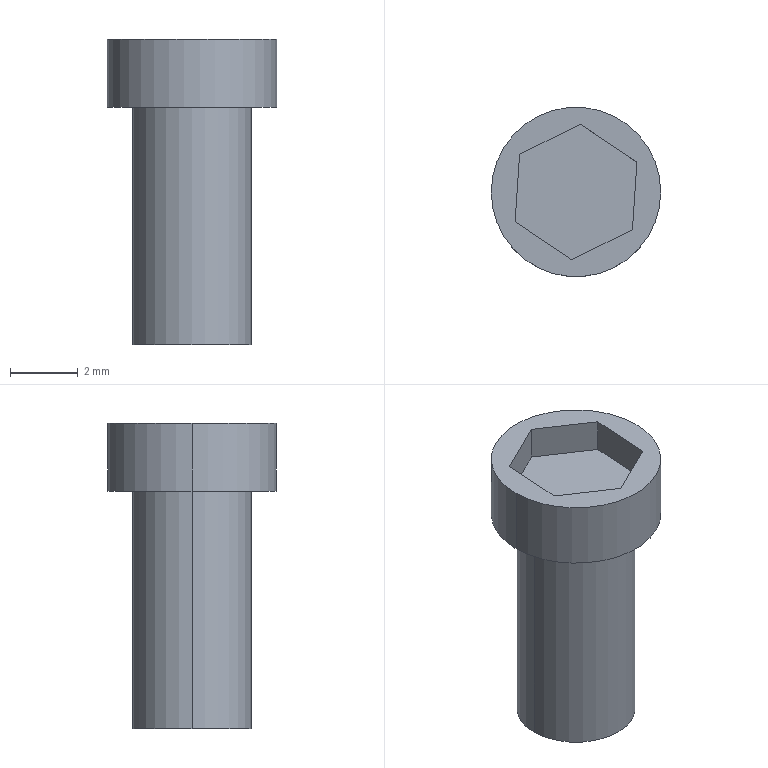Part | SolidWorks | features ICE 2, Extrusion 1 | 1 solid | 14 faces | box 5 x 5 x 9 mm | volume 96.197 mm3 | plane 10 | cylinder 4 | commonest cylinder face diameters 3.5 x2 5 x2
STEP:
#1=CARTESIAN_POINT('',(-1.75,0.,-7.));
#2=VERTEX_POINT('',#1);
#3=CARTESIAN_POINT('',(1.75,0.,-7.));
#4=VERTEX_POINT('',#3);
#5=CARTESIAN_POINT('',(0.,0.,-7.));
#6=DIRECTION('',(0.,0.,-1.));
#7=DIRECTION('',(-1.,0.,0.));
#8=AXIS2_PLACEMENT_3D('',#5,#6,#7);
#9=CIRCLE('',#8,1.75);
#10=EDGE_CURVE('',#2,#4,#9,.T.);
#11=ORIENTED_EDGE('',*,*,#10,.F.);
#12=CARTESIAN_POINT('',(-1.75,0.,0.));
#13=VERTEX_POINT('',#12);
#14=CARTESIAN_POINT('',(-1.75,0.,-7.));
#15=DIRECTION('',(0.,0.,1.));
#16=VECTOR('',#15,1000.);
#17=LINE('',#14,#16);
#18=EDGE_CURVE('',#2,#13,#17,.T.);
#19=ORIENTED_EDGE('',*,*,#18,.T.);
#20=CARTESIAN_POINT('',(1.75,0.,0.));
#21=VERTEX_POINT('',#20);
#22=CARTESIAN_POINT('',(0.,0.,0.));
#23=DIRECTION('',(0.,0.,-1.));
#24=DIRECTION('',(-1.,0.,0.));
#25=AXIS2_PLACEMENT_3D('',#22,#23,#24);
#26=CIRCLE('',#25,1.75);
#27=EDGE_CURVE('',#13,#21,#26,.T.);
#28=ORIENTED_EDGE('',*,*,#27,.T.);
#29=CARTESIAN_POINT('',(1.75,0.,-7.));
#30=DIRECTION('',(0.,0.,1.));
#31=VECTOR('',#30,1000.);
#32=LINE('',#29,#31);
#33=EDGE_CURVE('',#4,#21,#32,.T.);
#34=ORIENTED_EDGE('',*,*,#33,.F.);
#35=EDGE_LOOP('',(#11,#19,#28,#34));
#36=FACE_OUTER_BOUND('',#35,.T.);
#37=CARTESIAN_POINT('',(0.,0.,-7.));
#38=DIRECTION('',(0.,0.,1.));
#39=DIRECTION('',(1.,0.,0.));
#40=AXIS2_PLACEMENT_3D('',#37,#38,#39);
#41=CYLINDRICAL_SURFACE('',#40,1.75);
#42=ADVANCED_FACE('',(#36),#41,.T.);
#43=CARTESIAN_POINT('',(2.5,0.,2.));
#44=VERTEX_POINT('',#43);
#45=CARTESIAN_POINT('',(-2.5,0.,2.));
#46=VERTEX_POINT('',#45);
#47=CARTESIAN_POINT('',(0.,0.,2.));
#48=DIRECTION('',(0.,0.,1.));
#49=DIRECTION('',(1.,0.,0.));
#50=AXIS2_PLACEMENT_3D('',#47,#48,#49);
#51=CIRCLE('',#50,2.5);
#52=EDGE_CURVE('',#44,#46,#51,.T.);
#53=ORIENTED_EDGE('',*,*,#52,.F.);
#54=CARTESIAN_POINT('',(2.5,0.,0.));
#55=VERTEX_POINT('',#54);
#56=CARTESIAN_POINT('',(2.5,0.,2.));
#57=DIRECTION('',(0.,0.,-1.));
#58=VECTOR('',#57,1000.);
#59=LINE('',#56,#58);
#60=EDGE_CURVE('',#44,#55,#59,.T.);
#61=ORIENTED_EDGE('',*,*,#60,.T.);
#62=CARTESIAN_POINT('',(-2.5,0.,0.));
#63=VERTEX_POINT('',#62);
#64=CARTESIAN_POINT('',(0.,0.,0.));
#65=DIRECTION('',(0.,0.,1.));
#66=DIRECTION('',(1.,0.,0.));
#67=AXIS2_PLACEMENT_3D('',#64,#65,#66);
#68=CIRCLE('',#67,2.5);
#69=EDGE_CURVE('',#55,#63,#68,.T.);
#70=ORIENTED_EDGE('',*,*,#69,.T.);
#71=CARTESIAN_POINT('',(-2.5,0.,2.));
#72=DIRECTION('',(0.,0.,-1.));
#73=VECTOR('',#72,1000.);
#74=LINE('',#71,#73);
#75=EDGE_CURVE('',#46,#63,#74,.T.);
#76=ORIENTED_EDGE('',*,*,#75,.F.);
#77=EDGE_LOOP('',(#53,#61,#70,#76));
#78=FACE_OUTER_BOUND('',#77,.T.);
#79=CARTESIAN_POINT('',(0.,0.,2.));
#80=DIRECTION('',(0.,0.,-1.));
#81=DIRECTION('',(-1.,0.,0.));
#82=AXIS2_PLACEMENT_3D('',#79,#80,#81);
#83=CYLINDRICAL_SURFACE('',#82,2.5);
#84=ADVANCED_FACE('',(#78),#83,.T.);
#85=ORIENTED_EDGE('',*,*,#60,.F.);
#86=CARTESIAN_POINT('',(0.,0.,2.));
#87=DIRECTION('',(0.,0.,1.));
#88=DIRECTION('',(1.,0.,0.));
#89=AXIS2_PLACEMENT_3D('',#86,#87,#88);
#90=CIRCLE('',#89,2.5);
#91=EDGE_CURVE('',#46,#44,#90,.T.);
#92=ORIENTED_EDGE('',*,*,#91,.F.);
#93=ORIENTED_EDGE('',*,*,#75,.T.);
#94=CARTESIAN_POINT('',(0.,0.,0.));
#95=DIRECTION('',(0.,0.,1.));
#96=DIRECTION('',(1.,0.,0.));
#97=AXIS2_PLACEMENT_3D('',#94,#95,#96);
#98=CIRCLE('',#97,2.5);
#99=EDGE_CURVE('',#63,#55,#98,.T.);
#100=ORIENTED_EDGE('',*,*,#99,.T.);
#101=EDGE_LOOP('',(#85,#92,#93,#100));
#102=FACE_OUTER_BOUND('',#101,.T.);
#103=CARTESIAN_POINT('',(0.,0.,2.));
#104=DIRECTION('',(0.,0.,-1.));
#105=DIRECTION('',(-1.,0.,0.));
#106=AXIS2_PLACEMENT_3D('',#103,#104,#105);
#107=CYLINDRICAL_SURFACE('',#106,2.5);
#108=ADVANCED_FACE('',(#102),#107,.T.);
#109=CARTESIAN_POINT('',(-0.1337,-1.998,2.));
#110=VERTEX_POINT('',#109);
#111=CARTESIAN_POINT('',(1.664,-1.115,2.));
#112=VERTEX_POINT('',#111);
#113=CARTESIAN_POINT('',(-0.1337,-1.998,2.));
#114=DIRECTION('',(0.8975,0.4411,0.));
#115=VECTOR('',#114,1000.);
#116=LINE('',#113,#115);
#117=EDGE_CURVE('',#110,#112,#116,.T.);
#118=ORIENTED_EDGE('',*,*,#117,.F.);
#119=CARTESIAN_POINT('',(-1.797,-0.8833,2.));
#120=VERTEX_POINT('',#119);
#121=CARTESIAN_POINT('',(-1.797,-0.8833,2.));
#122=DIRECTION('',(0.8307,-0.5567,0.));
#123=VECTOR('',#122,1000.);
#124=LINE('',#121,#123);
#125=EDGE_CURVE('',#120,#110,#124,.T.);
#126=ORIENTED_EDGE('',*,*,#125,.F.);
#127=CARTESIAN_POINT('',(-1.664,1.115,2.));
#128=VERTEX_POINT('',#127);
#129=CARTESIAN_POINT('',(-1.664,1.115,2.));
#130=DIRECTION('',(-0.06677,-0.9978,0.));
#131=VECTOR('',#130,1000.);
#132=LINE('',#129,#131);
#133=EDGE_CURVE('',#128,#120,#132,.T.);
#134=ORIENTED_EDGE('',*,*,#133,.F.);
#135=CARTESIAN_POINT('',(0.1337,1.998,2.));
#136=VERTEX_POINT('',#135);
#137=CARTESIAN_POINT('',(0.1337,1.998,2.));
#138=DIRECTION('',(-0.8975,-0.4411,0.));
#139=VECTOR('',#138,1000.);
#140=LINE('',#137,#139);
#141=EDGE_CURVE('',#136,#128,#140,.T.);
#142=ORIENTED_EDGE('',*,*,#141,.F.);
#143=CARTESIAN_POINT('',(1.797,0.8833,2.));
#144=VERTEX_POINT('',#143);
#145=CARTESIAN_POINT('',(1.797,0.8833,2.));
#146=DIRECTION('',(-0.8307,0.5567,0.));
#147=VECTOR('',#146,1000.);
#148=LINE('',#145,#147);
#149=EDGE_CURVE('',#144,#136,#148,.T.);
#150=ORIENTED_EDGE('',*,*,#149,.F.);
#151=CARTESIAN_POINT('',(1.664,-1.115,2.));
#152=DIRECTION('',(0.06677,0.9978,0.));
#153=VECTOR('',#152,1000.);
#154=LINE('',#151,#153);
#155=EDGE_CURVE('',#112,#144,#154,.T.);
#156=ORIENTED_EDGE('',*,*,#155,.F.);
#157=EDGE_LOOP('',(#118,#126,#134,#142,#150,#156));
#158=FACE_BOUND('',#157,.T.);
#159=ORIENTED_EDGE('',*,*,#91,.T.);
#160=ORIENTED_EDGE('',*,*,#52,.T.);
#161=EDGE_LOOP('',(#159,#160));
#162=FACE_OUTER_BOUND('',#161,.T.);
#163=CARTESIAN_POINT('',(0.,0.,2.));
#164=DIRECTION('',(0.,0.,1.));
#165=DIRECTION('',(1.,0.,0.));
#166=AXIS2_PLACEMENT_3D('',#163,#164,#165);
#167=PLANE('',#166);
#168=ADVANCED_FACE('',(#158,#162),#167,.T.);
#169=CARTESIAN_POINT('',(0.,0.,0.));
#170=DIRECTION('',(0.,0.,-1.));
#171=DIRECTION('',(-1.,0.,0.));
#172=AXIS2_PLACEMENT_3D('',#169,#170,#171);
#173=CIRCLE('',#172,1.75);
#174=EDGE_CURVE('',#21,#13,#173,.T.);
#175=ORIENTED_EDGE('',*,*,#174,.F.);
#176=ORIENTED_EDGE('',*,*,#27,.F.);
#177=EDGE_LOOP('',(#175,#176));
#178=FACE_BOUND('',#177,.T.);
#179=ORIENTED_EDGE('',*,*,#99,.F.);
#180=ORIENTED_EDGE('',*,*,#69,.F.);
#181=EDGE_LOOP('',(#179,#180));
#182=FACE_OUTER_BOUND('',#181,.T.);
#183=CARTESIAN_POINT('',(0.,0.,0.));
#184=DIRECTION('',(0.,0.,1.));
#185=DIRECTION('',(1.,0.,0.));
#186=AXIS2_PLACEMENT_3D('',#183,#184,#185);
#187=PLANE('',#186);
#188=ADVANCED_FACE('',(#178,#182),#187,.F.);
#189=ORIENTED_EDGE('',*,*,#117,.T.);
#190=CARTESIAN_POINT('',(1.664,-1.115,1.));
#191=VERTEX_POINT('',#190);
#192=CARTESIAN_POINT('',(1.664,-1.115,1.));
#193=DIRECTION('',(0.,0.,1.));
#194=VECTOR('',#193,1000.);
#195=LINE('',#192,#194);
#196=EDGE_CURVE('',#191,#112,#195,.T.);
#197=ORIENTED_EDGE('',*,*,#196,.F.);
#198=CARTESIAN_POINT('',(-0.1337,-1.998,1.));
#199=VERTEX_POINT('',#198);
#200=CARTESIAN_POINT('',(-0.1337,-1.998,1.));
#201=DIRECTION('',(0.8975,0.4411,0.));
#202=VECTOR('',#201,1000.);
#203=LINE('',#200,#202);
#204=EDGE_CURVE('',#199,#191,#203,.T.);
#205=ORIENTED_EDGE('',*,*,#204,.F.);
#206=CARTESIAN_POINT('',(-0.1337,-1.998,1.));
#207=DIRECTION('',(0.,0.,1.));
#208=VECTOR('',#207,1000.);
#209=LINE('',#206,#208);
#210=EDGE_CURVE('',#199,#110,#209,.T.);
#211=ORIENTED_EDGE('',*,*,#210,.T.);
#212=EDGE_LOOP('',(#189,#197,#205,#211));
#213=FACE_OUTER_BOUND('',#212,.T.);
#214=CARTESIAN_POINT('',(-0.1337,-1.998,1.));
#215=DIRECTION('',(0.4411,-0.8975,0.));
#216=DIRECTION('',(0.8975,0.4411,0.));
#217=AXIS2_PLACEMENT_3D('',#214,#215,#216);
#218=PLANE('',#217);
#219=ADVANCED_FACE('',(#213),#218,.F.);
#220=ORIENTED_EDGE('',*,*,#125,.T.);
#221=ORIENTED_EDGE('',*,*,#210,.F.);
#222=CARTESIAN_POINT('',(-1.797,-0.8833,1.));
#223=VERTEX_POINT('',#222);
#224=CARTESIAN_POINT('',(-1.797,-0.8833,1.));
#225=DIRECTION('',(0.8307,-0.5567,0.));
#226=VECTOR('',#225,1000.);
#227=LINE('',#224,#226);
#228=EDGE_CURVE('',#223,#199,#227,.T.);
#229=ORIENTED_EDGE('',*,*,#228,.F.);
#230=CARTESIAN_POINT('',(-1.797,-0.8833,1.));
#231=DIRECTION('',(0.,0.,1.));
#232=VECTOR('',#231,1000.);
#233=LINE('',#230,#232);
#234=EDGE_CURVE('',#223,#120,#233,.T.);
#235=ORIENTED_EDGE('',*,*,#234,.T.);
#236=EDGE_LOOP('',(#220,#221,#229,#235));
#237=FACE_OUTER_BOUND('',#236,.T.);
#238=CARTESIAN_POINT('',(-1.797,-0.8833,1.));
#239=DIRECTION('',(-0.5567,-0.8307,0.));
#240=DIRECTION('',(0.8307,-0.5567,0.));
#241=AXIS2_PLACEMENT_3D('',#238,#239,#240);
#242=PLANE('',#241);
#243=ADVANCED_FACE('',(#237),#242,.F.);
#244=ORIENTED_EDGE('',*,*,#133,.T.);
#245=ORIENTED_EDGE('',*,*,#234,.F.);
#246=CARTESIAN_POINT('',(-1.664,1.115,1.));
#247=VERTEX_POINT('',#246);
#248=CARTESIAN_POINT('',(-1.664,1.115,1.));
#249=DIRECTION('',(-0.06677,-0.9978,0.));
#250=VECTOR('',#249,1000.);
#251=LINE('',#248,#250);
#252=EDGE_CURVE('',#247,#223,#251,.T.);
#253=ORIENTED_EDGE('',*,*,#252,.F.);
#254=CARTESIAN_POINT('',(-1.664,1.115,1.));
#255=DIRECTION('',(0.,0.,1.));
#256=VECTOR('',#255,1000.);
#257=LINE('',#254,#256);
#258=EDGE_CURVE('',#247,#128,#257,.T.);
#259=ORIENTED_EDGE('',*,*,#258,.T.);
#260=EDGE_LOOP('',(#244,#245,#253,#259));
#261=FACE_OUTER_BOUND('',#260,.T.);
#262=CARTESIAN_POINT('',(-1.664,1.115,1.));
#263=DIRECTION('',(-0.9978,0.06677,0.));
#264=DIRECTION('',(-0.06677,-0.9978,0.));
#265=AXIS2_PLACEMENT_3D('',#262,#263,#264);
#266=PLANE('',#265);
#267=ADVANCED_FACE('',(#261),#266,.F.);
#268=ORIENTED_EDGE('',*,*,#141,.T.);
#269=ORIENTED_EDGE('',*,*,#258,.F.);
#270=CARTESIAN_POINT('',(0.1337,1.998,1.));
#271=VERTEX_POINT('',#270);
#272=CARTESIAN_POINT('',(0.1337,1.998,1.));
#273=DIRECTION('',(-0.8975,-0.4411,0.));
#274=VECTOR('',#273,1000.);
#275=LINE('',#272,#274);
#276=EDGE_CURVE('',#271,#247,#275,.T.);
#277=ORIENTED_EDGE('',*,*,#276,.F.);
#278=CARTESIAN_POINT('',(0.1337,1.998,1.));
#279=DIRECTION('',(0.,0.,1.));
#280=VECTOR('',#279,1000.);
#281=LINE('',#278,#280);
#282=EDGE_CURVE('',#271,#136,#281,.T.);
#283=ORIENTED_EDGE('',*,*,#282,.T.);
#284=EDGE_LOOP('',(#268,#269,#277,#283));
#285=FACE_OUTER_BOUND('',#284,.T.);
#286=CARTESIAN_POINT('',(0.1337,1.998,1.));
#287=DIRECTION('',(-0.4411,0.8975,0.));
#288=DIRECTION('',(-0.8975,-0.4411,0.));
#289=AXIS2_PLACEMENT_3D('',#286,#287,#288);
#290=PLANE('',#289);
#291=ADVANCED_FACE('',(#285),#290,.F.);
#292=ORIENTED_EDGE('',*,*,#149,.T.);
#293=ORIENTED_EDGE('',*,*,#282,.F.);
#294=CARTESIAN_POINT('',(1.797,0.8833,1.));
#295=VERTEX_POINT('',#294);
#296=CARTESIAN_POINT('',(1.797,0.8833,1.));
#297=DIRECTION('',(-0.8307,0.5567,0.));
#298=VECTOR('',#297,1000.);
#299=LINE('',#296,#298);
#300=EDGE_CURVE('',#295,#271,#299,.T.);
#301=ORIENTED_EDGE('',*,*,#300,.F.);
#302=CARTESIAN_POINT('',(1.797,0.8833,1.));
#303=DIRECTION('',(0.,0.,1.));
#304=VECTOR('',#303,1000.);
#305=LINE('',#302,#304);
#306=EDGE_CURVE('',#295,#144,#305,.T.);
#307=ORIENTED_EDGE('',*,*,#306,.T.);
#308=EDGE_LOOP('',(#292,#293,#301,#307));
#309=FACE_OUTER_BOUND('',#308,.T.);
#310=CARTESIAN_POINT('',(1.797,0.8833,1.));
#311=DIRECTION('',(0.5567,0.8307,0.));
#312=DIRECTION('',(-0.8307,0.5567,0.));
#313=AXIS2_PLACEMENT_3D('',#310,#311,#312);
#314=PLANE('',#313);
#315=ADVANCED_FACE('',(#309),#314,.F.);
#316=ORIENTED_EDGE('',*,*,#155,.T.);
#317=ORIENTED_EDGE('',*,*,#306,.F.);
#318=CARTESIAN_POINT('',(1.664,-1.115,1.));
#319=DIRECTION('',(0.06677,0.9978,0.));
#320=VECTOR('',#319,1000.);
#321=LINE('',#318,#320);
#322=EDGE_CURVE('',#191,#295,#321,.T.);
#323=ORIENTED_EDGE('',*,*,#322,.F.);
#324=ORIENTED_EDGE('',*,*,#196,.T.);
#325=EDGE_LOOP('',(#316,#317,#323,#324));
#326=FACE_OUTER_BOUND('',#325,.T.);
#327=CARTESIAN_POINT('',(1.664,-1.115,1.));
#328=DIRECTION('',(0.9978,-0.06677,0.));
#329=DIRECTION('',(0.06677,0.9978,0.));
#330=AXIS2_PLACEMENT_3D('',#327,#328,#329);
#331=PLANE('',#330);
#332=ADVANCED_FACE('',(#326),#331,.F.);
#333=ORIENTED_EDGE('',*,*,#204,.T.);
#334=ORIENTED_EDGE('',*,*,#322,.T.);
#335=ORIENTED_EDGE('',*,*,#300,.T.);
#336=ORIENTED_EDGE('',*,*,#276,.T.);
#337=ORIENTED_EDGE('',*,*,#252,.T.);
#338=ORIENTED_EDGE('',*,*,#228,.T.);
#339=EDGE_LOOP('',(#333,#334,#335,#336,#337,#338));
#340=FACE_OUTER_BOUND('',#339,.T.);
#341=CARTESIAN_POINT('',(0.,0.,1.));
#342=DIRECTION('',(0.,0.,1.));
#343=DIRECTION('',(1.,0.,0.));
#344=AXIS2_PLACEMENT_3D('',#341,#342,#343);
#345=PLANE('',#344);
#346=ADVANCED_FACE('',(#340),#345,.T.);
#347=ORIENTED_EDGE('',*,*,#18,.F.);
#348=CARTESIAN_POINT('',(0.,0.,-7.));
#349=DIRECTION('',(0.,0.,-1.));
#350=DIRECTION('',(-1.,0.,0.));
#351=AXIS2_PLACEMENT_3D('',#348,#349,#350);
#352=CIRCLE('',#351,1.75);
#353=EDGE_CURVE('',#4,#2,#352,.T.);
#354=ORIENTED_EDGE('',*,*,#353,.F.);
#355=ORIENTED_EDGE('',*,*,#33,.T.);
#356=ORIENTED_EDGE('',*,*,#174,.T.);
#357=EDGE_LOOP('',(#347,#354,#355,#356));
#358=FACE_OUTER_BOUND('',#357,.T.);
#359=CARTESIAN_POINT('',(0.,0.,-7.));
#360=DIRECTION('',(0.,0.,1.));
#361=DIRECTION('',(1.,0.,0.));
#362=AXIS2_PLACEMENT_3D('',#359,#360,#361);
#363=CYLINDRICAL_SURFACE('',#362,1.75);
#364=ADVANCED_FACE('',(#358),#363,.T.);
#365=ORIENTED_EDGE('',*,*,#353,.T.);
#366=ORIENTED_EDGE('',*,*,#10,.T.);
#367=EDGE_LOOP('',(#365,#366));
#368=FACE_OUTER_BOUND('',#367,.T.);
#369=CARTESIAN_POINT('',(0.,0.,-7.));
#370=DIRECTION('',(0.,0.,-1.));
#371=DIRECTION('',(-1.,0.,0.));
#372=AXIS2_PLACEMENT_3D('',#369,#370,#371);
#373=PLANE('',#372);
#374=ADVANCED_FACE('',(#368),#373,.T.);
#375=CLOSED_SHELL('',(#42,#84,#108,#168,#188,#219,#243,#267,#291,#315,#332,#346,#364,#374));
#376=MANIFOLD_SOLID_BREP('',#375);
#377=CARTESIAN_POINT('',(0.,0.,0.));
#378=DIRECTION('',(0.,0.,1.));
#379=DIRECTION('',(1.,0.,0.));
#380=AXIS2_PLACEMENT_3D('',#377,#378,#379);
#381=(LENGTH_UNIT()NAMED_UNIT(*)SI_UNIT(.MILLI.,.METRE.));
#382=UNCERTAINTY_MEASURE_WITH_UNIT(LENGTH_MEASURE(0.00001),#381,'','');
#383=(NAMED_UNIT(*)PLANE_ANGLE_UNIT()SI_UNIT($,.RADIAN.));
#384=(NAMED_UNIT(*)SI_UNIT($,.STERADIAN.)SOLID_ANGLE_UNIT());
#385=(GEOMETRIC_REPRESENTATION_CONTEXT(3)GLOBAL_UNCERTAINTY_ASSIGNED_CONTEXT((#382))GLOBAL_UNIT_ASSIGNED_CONTEXT((#381,#383,#384))REPRESENTATION_CONTEXT('',''));
#386=ADVANCED_BREP_SHAPE_REPRESENTATION('',(#376,#380),#385);